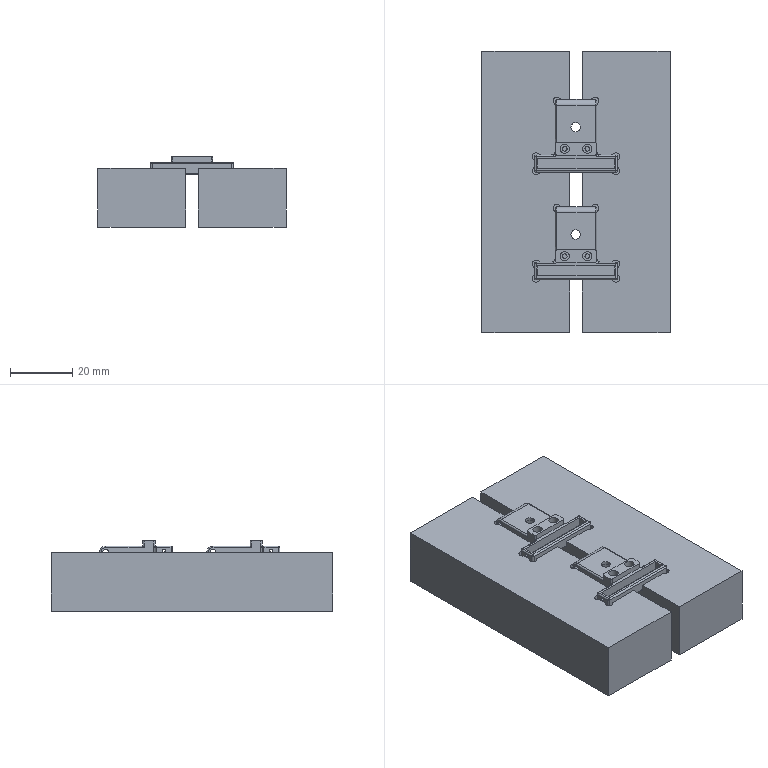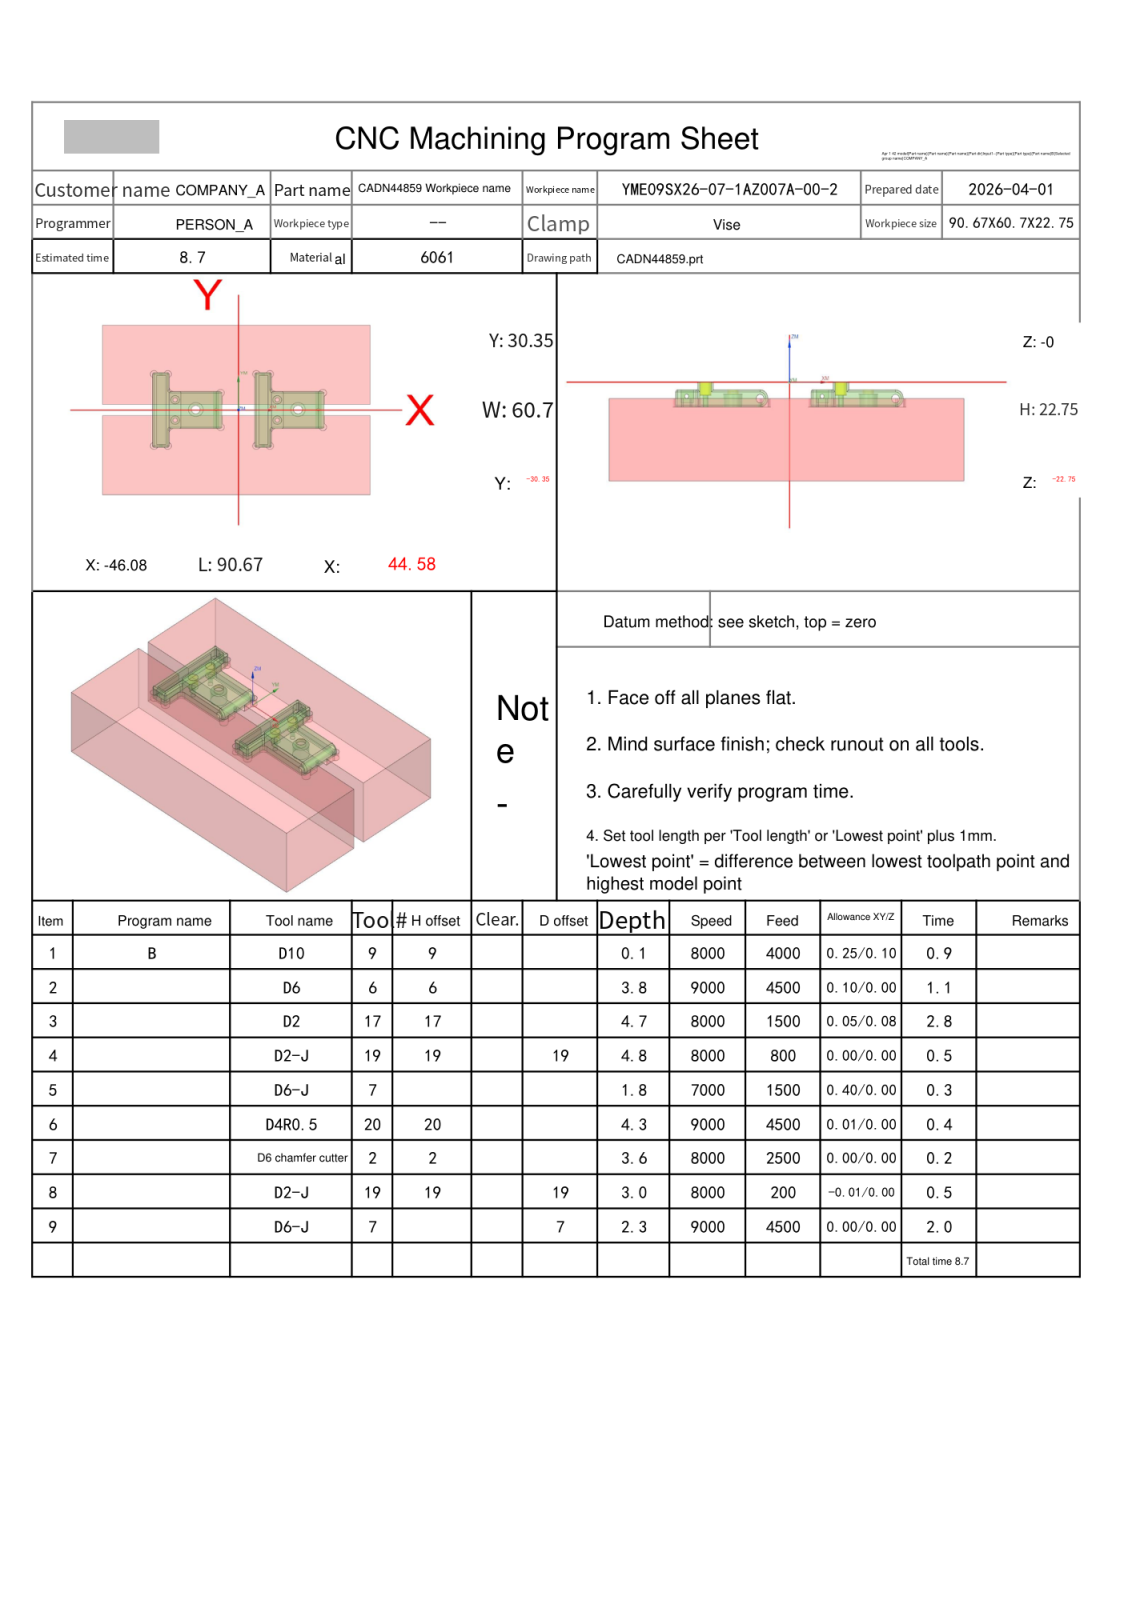NC program | NX | posted by the shop | part box 60.696 x 90.669 x 22.754 mm
Lines 1 to 1599 of 6042:
%
O0001
(Machine time: 10.48 MIN)
(===Total Tool:7===)
(T9=D10     D=10.  R=0.   D-  H09 Z=0.1   )
(T6=D6      D=6.   R=0.   D-  H06 Z=-3.79 )
(T17=D2     D=2.   R=0.   D-  H17 Z=-4.69 )
(T19=D2-J   D=2.   R=0.   D19 H19 Z=-4.75 )
(T7=D6-J    D=6.   R=0.   D-  H00 Z=-2.25 )
(T20=D4R0.5 D=4.   R=0.5  D-  H20 Z=-4.29 )
(T2=D6 chamfer cutter   D=6.   R=0.   D-  H02 Z=-3.55 )
G80 G90 G17 G49 G40
G91 G28 Z0
M01
N1 T09 M06
(D10  D=10. R=0. H=09 ce=0.25 di=0.10)
G00 G90 G54 X-40.842 Y20.381 M03 S8000
G43 H09 Z20.
M08
Z2.1
G01 X-40.747 Y20.349 Z1.476 F4000.
X-40.652 Y20.318 Z1.228
X-40.557 Y20.286 Z1.046
X-40.463 Y20.254 Z.9
X-40.368 Y20.222 Z.777
X-40.273 Y20.19 Z.672
X-40.178 Y20.158 Z.58
X-40.083 Y20.126 Z.5
X-39.989 Y20.094 Z.43
X-39.894 Y20.062 Z.368
X-39.799 Y20.03 Z.314
X-39.704 Y19.999 Z.267
X-39.61 Y19.967 Z.227
X-39.515 Y19.935 Z.192
X-39.42 Y19.903 Z.164
X-39.325 Y19.871 Z.14
X-39.23 Y19.839 Z.123
X-39.136 Y19.807 Z.11
X-39.041 Y19.775 Z.103
X-38.946 Y19.743 Z.1
X-36.729 Y18.997
X-36.569 Y18.972
G03 X-36.315 Y19.038 I0.0 J.518
G02 X-33.516 Y19.957 I3.756 J-6.724
X-26.927 Y20.43 I6.589 J-45.637
X-26.22 Y20.425 I0.0 J-46.111
G01 X30.138 Y20.424
G02 X36.151 Y16.155 I-.263 J-6.74
X37.336 Y10.243 I-16.003 J-6.282
X37.502 Y.85 I-265.863 J-9.393
X37.485 Y-2.174 I-266.029 J0.0
X37.502 Y-6.249 I-476.949 J-4.074
X37.45 Y-13.253 I-476.966 J0.0
X33.27 Y-19.077 I-6.701 J.398
X27.726 Y-20.269 I-6.122 J14.98
X19.91 Y-20.455 I-7.816 J164.512
X18.189 Y-20.446 I0.0 J164.698
G01 X-30.028 Y-20.429
G02 X-36.161 Y-16.157 I.154 J6.76
X-37.332 Y-10.366 I15.734 J6.194
X-37.505 Y-.549 I277.888 J9.817
X-37.485 Y2.832 I278.061 J0.0
X-37.5 Y6.556 I451.277 J3.724
X-37.452 Y13.13 I451.292 J0.0
X-34.138 Y17.894 I6.402 J-.919
X-28.596 Y19.537 I6.567 J-11.986
X-20.913 Y19.853 I7.683 J-93.113
X-19.426 Y19.842 I0.0 J-93.429
G01 X28.403 Y19.826
G02 X35.029 Y15.447 I-.346 J-7.726
X36.613 Y9.328 I-14.784 J-7.091
X36.901 Y.457 I-136.295 J-8.871
X36.882 Y-1.825 I-136.584 J0.0
X36.903 Y-5.413 I-318.323 J-3.588
X36.84 Y-11.719 I-318.344 J0.0
X32.586 Y-17.937 I-7.685 J.693
X26.481 Y-19.565 I-7.111 J14.409
X18.572 Y-19.851 I-7.909 J109.299
X17.188 Y-19.842 I0.0 J109.585
G01 X-28.373 Y-19.827
G02 X-35.024 Y-15.475 I.301 J7.717
X-36.614 Y-9.353 I14.682 J7.081
X-36.897 Y-.811 I128.482 J8.542
X-36.882 Y1.2 I128.765 J0.0
X-36.896 Y4.786 I434.55 J3.585
X-36.851 Y11.095 I434.565 J0.0
X-32.53 Y17.279 I7.805 J-.852
X-26.194 Y18.96 I7.343 J-14.892
X-17.308 Y19.262 I8.886 J-130.709
X-15.161 Y19.244 I0.0 J-131.01
G01 X26.759 Y19.226
G02 X34.346 Y14.205 I-.291 J-8.684
X36.01 Y7.485 I-16.807 J-7.728
X36.295 Y-1.458 I-140.358 J-8.942
X36.281 Y-3.429 I-140.642 J0.0
X36.305 Y-5.816 I-120.556 J-2.387
X36.22 Y-10.327 I-120.58 J0.0
X31.284 Y-17.288 I-8.629 J.888
X24.694 Y-18.957 I-7.673 J16.445
X16.023 Y-19.254 I-8.671 J126.585
X14.321 Y-19.243 I0.0 J126.881
G01 X-26.819 Y-19.224
G02 X-34.337 Y-14.236 I.331 J8.66
X-35.987 Y-7.756 I16.355 J7.615
X-36.287 Y.642 I117.427 J8.398
X-36.278 Y2.077 I117.726 J0.0
X-36.296 Y4.741 I199.73 J2.664
X-36.24 Y9.456 I199.747 J0.0
X-31.263 Y16.631 I8.743 J-.75
X-24.498 Y18.353 I7.851 J-16.702
X-15.886 Y18.651 I8.612 J-124.221
X-14.365 Y18.641 I0.0 J-124.519
G01 X25.094 Y18.63
G02 X33.792 Y12.869 I-.033 J-9.496
X35.393 Y6.07 I-18.671 J-7.984
X35.689 Y-2.856 I-134.771 J-8.926
X35.679 Y-4.483 I-135.066 J0.0
X35.704 Y-5.918 I-41.196 J-1.435
X35.557 Y-9.398 I-41.22 J0.0
X30.113 Y-16.656 I-9.314 J1.315
X23.151 Y-18.352 I-8.101 J18.111
X13.766 Y-18.658 I-9.385 J143.679
X11.698 Y-18.643 I0.0 J143.985
G01 X-25.181 Y-18.627
G02 X-33.711 Y-13.049 I.086 J9.443
X-35.383 Y-6.202 I18.062 J8.037
X-35.69 Y2.818 I132.251 J9.019
X-35.679 Y4.531 I132.558 J0.0
X-35.706 Y5.721 I26.507 J1.19
X-35.477 Y9.199 I26.534 J0.0
X-29.991 Y16.061 I9.358 J-1.857
X-22.967 Y17.751 I8.183 J-18.58
X-13.276 Y18.06 I9.691 J-151.435
X-11.034 Y18.044 I0.0 J-151.744
G01 X23.746 Y18.025
X23.806
G02 X33.198 Y11.714 I0.0 J-10.144
X34.785 Y4.722 I-20.248 J-8.273
X35.081 Y-3.446 I-112.509 J-8.168
X35.006 Y-7.569 I-112.805 J0.0
X29.038 Y-16.028 I-9.98 J.707
X21.957 Y-17.731 I-8.374 J19.249
X12.963 Y-18.047 I-8.995 J127.82
X11.585 Y-18.039 I0.0 J128.136
G01 X-23.854 Y-18.021
G02 X-33.178 Y-11.765 I.026 J10.114
X-34.792 Y-4.658 I20.204 J8.325
X-35.08 Y2.895 I98.916 J7.553
X-34.996 Y6.973 I99.204 J0.0
X-28.872 Y15.46 I10.08 J-.82
X-21.542 Y17.153 I8.509 J-20.134
X-11.764 Y17.457 I9.779 J-156.976
X-9.669 Y17.443 I0.0 J-157.28
G01 X22.411 Y17.423
X22.526 Y17.424
G02 X29.094 Y15.286 I0.0 J-11.159
X33.223 Y8.914 I-7.735 J-9.536
X34.333 Y1.092 I-31.665 J-8.482
X34.457 Y-3.082 I-70.23 J-4.174
X34.37 Y-6.584 I-70.354 J0.0
X28.073 Y-15.382 I-10.446 J.824
X20.694 Y-17.126 I-8.701 J20.336
X11.245 Y-17.449 I-9.449 J138.124
X9.662 Y-17.44 I0.0 J138.447
G01 X-22.298 Y-17.427
X-22.478 Y-17.429
G02 X-28.767 Y-15.53 I0.0 J11.362
X-33.17 Y-9.095 I7.176 J9.635
X-34.322 Y-1.341 I30.345 J8.469
X-34.448 Y2.658 I63.448 J4.
X-34.365 Y5.914 I63.574 J0.0
X-28.047 Y14.754 I10.508 J-.832
X-20.613 Y16.52 I8.772 J-20.399
X-10.524 Y16.857 I10.09 J-150.833
X-8.381 Y16.842 I0.0 J-151.17
G01 X21.119 Y16.823
X21.27 Y16.824
G02 X27.481 Y15.15 I0.0 J-12.36
X32.329 Y8.76 I-6.554 J-10.007
X33.685 Y.738 I-28.136 J-8.88
X33.821 Y-2.613 I-40.982 J-3.351
X33.674 Y-6.094 I-41.118 J0.0
X27.147 Y-14.745 I-10.767 J1.336
X19.709 Y-16.503 I-8.893 J21.002
X9.271 Y-16.859 I-10.437 J153.067
X6.997 Y-16.842 I0.0 J153.422
G01 X-21.123 Y-16.823
X-21.282 Y-16.824
G02 X-27.535 Y-15.119 I0.0 J12.32
X-32.372 Y-8.644 I6.661 J10.019
X-33.689 Y-.677 I28.655 J8.828
X-33.81 Y2.187 I33.686 J2.863
X-33.63 Y5.673 I33.807 J0.0
X-27.198 Y14.086 I10.766 J-1.566
X-19.887 Y15.875 I8.898 J-20.532
X-10.326 Y16.243 I9.56 J-123.703
X-8.976 Y16.236 I0.0 J-124.071
G01 X19.803 Y16.225
G02 X20.034 Y16.227 I.231 J-13.722
X26.069 Y14.829 I0.0 J-13.723
X31.497 Y8.398 I-5.798 J-10.401
X33.02 Y.534 I-25.713 J-9.06
X33.162 Y-2.216 I-26.672 J-2.75
X32.92 Y-5.81 I-26.814 J0.0
X26.456 Y-14.017 I-10.93 J1.96
X18.737 Y-15.886 I-9.21 J21.158
X9.038 Y-16.243 I-9.699 J131.666
X7.706 Y-16.236 I0.0 J132.023
G01 X-19.814 Y-16.225
G02 X-20.043 Y-16.227 I-.229 J13.682
X-26.131 Y-14.798 I0.0 J13.684
X-31.549 Y-8.27 I5.907 J10.415
X-33.034 Y-.337 I26.359 J9.04
X-33.145 Y1.84 I21.233 J2.177
X-32.783 Y5.756 I21.344 J0.0
X-26.29 Y13.463 I10.887 J-2.584
X-18.682 Y15.281 I9.163 J-21.514
X-8.617 Y15.648 I10.065 J-137.713
X-6.931 Y15.638 I0.0 J-138.081
G01 X18.788 Y15.62
X18.969 Y15.621
G02 X25.076 Y14.274 I0.0 J-14.52
X30.864 Y7.541 I-5.713 J-10.764
X32.445 Y-1.785 I-26.711 J-9.326
X32.319 Y-4.455 I-28.292 J0.0
X25.681 Y-13.343 I-11.223 J1.459
X17.911 Y-15.26 I-9.381 J21.327
X7.488 Y-15.651 I-10.423 J138.606
X5.621 Y-15.638 I0.0 J138.997
G01 X-18.539 Y-15.627
G02 X-18.83 Y-15.63 I-.291 J15.256
X-24.739 Y-14.439 I0.0 J15.259
X-30.735 Y-7.872 I5.218 J10.785
X-32.41 Y.927 I24.809 J9.282
X-32.444 Y1.868 I13.077 J.941
X-31.034 Y7.783 I13.111 J0.0
X-24.378 Y13.269 I10.606 J-6.087
X-16.207 Y14.792 I9.315 J-27.292
X-4.645 Y15.063 I11.563 J-246.703
X-1.572 Y15.044 I0.0 J-246.974
G01 X17.548 Y15.023
G02 X17.813 Y15.025 I.265 J-15.892
X23.925 Y13.803 I0.0 J-15.894
X30.063 Y7.135 I-5.288 J-11.028
X31.706 Y-1.466 I-21.699 J-8.601
X31.593 Y-3.761 I-23.341 J0.0
X24.903 Y-12.682 I-11.343 J1.537
X16.957 Y-14.649 I-9.592 J21.709
X6.501 Y-15.047 I-10.456 J137.135
X4.788 Y-15.037 I0.0 J137.533
G01 X-17.452 Y-15.025
G02 X-17.754 Y-15.028 I-.302 J16.286
X-23.73 Y-13.892 I0.0 J16.289
X-30.053 Y-7.166 I5.053 J11.085
X-31.652 Y.994 I20.017 J8.16
X-31.529 Y3.303 I21.616 J0.0
X-25.041 Y11.984 I11.274 J-1.661
X-17.35 Y13.999 I9.538 J-20.728
X-7.318 Y14.436 I10.032 J-114.813
X-6.143 Y14.43 I0.0 J-115.251
G01 X16.336 Y14.425
G02 X16.667 Y14.428 I.33 J-17.538
X22.69 Y13.361 I0.0 J-17.541
X29.351 Y6.525 I-4.821 J-11.36
X30.926 Y-1.13 I-17.821 J-7.655
X30.807 Y-3.277 I-19.396 J0.0
X24.37 Y-11.907 I-11.309 J1.72
X16.58 Y-13.982 I-9.682 J20.688
X6.084 Y-14.442 I-10.496 J119.566
X4.594 Y-14.433 I0.0 J120.025
G01 X-16.506 Y-14.421
G02 X-16.764 Y-14.423 I-.258 J17.012
X-22.847 Y-13.298 I0.0 J17.013
X-29.443 Y-6.312 I5.042 J11.367
X-30.855 Y.679 I16.599 J6.991
X-30.73 Y2.795 I18.011 J0.0
X-24.438 Y11.24 I11.232 J-1.802
X-16.843 Y13.341 I9.643 J-20.081
X-6.81 Y13.828 I10.033 J-103.144
X-5.879 Y13.824 I0.0 J-103.631
G01 X15.341 Y13.823
G02 X15.659 Y13.826 I.318 J-18.556
X21.707 Y12.813 I0.0 J-18.559
X28.697 Y5.798 I-4.657 J-11.63
X30.1 Y-.78 I-14.722 J-6.578
X29.938 Y-3.06 I-16.124 J0.0
X23.757 Y-11.17 I-11.184 J2.113
X15.879 Y-13.349 I-9.845 J20.262
X5.814 Y-13.827 I-10.066 J105.826
X4.975 Y-13.824 I0.0 J106.304
G01 X-15.345 Y-13.823
G02 X-15.682 Y-13.826 I-.337 J18.375
X-21.823 Y-12.77 I0.0 J18.378
X-28.784 Y-5.593 I4.808 J11.627
X-30.009 Y.306 I13.591 J5.899
X-29.796 Y2.807 I14.816 J0.0
X-23.736 Y10.548 I11.07 J-2.424
X-15.917 Y12.735 I9.838 J-20.102
X-5.509 Y13.233 I10.408 J-108.483
X-4.353 Y13.227 I0.0 J-108.981
X4.021 Y13.265 I8.374 J-925.635
X15.186 Y13.197 I0.0 J-925.673
G01 X15.195
G02 X21.944 Y11.749 I0.0 J-16.452
X28.374 Y4.22 I-5.943 J-11.585
X29.232 Y-.388 I-11.945 J-4.608
X28.738 Y-3.909 I-12.803 J0.0
X22.618 Y-10.704 I-10.949 J3.708
X14.879 Y-12.753 I-9.771 J21.262
X4.119 Y-13.239 I-10.761 J118.93
X2.654 Y-13.23 I0.0 J119.415
X-4.535 Y-13.262 I-7.189 J802.826
X-15.385 Y-13.189 I0.0 J802.858
X-22.226 Y-11.611 I.071 J15.92
X-28.521 Y-3.728 I6.265 J11.459
X-29.129 Y-.051 I10.82 J3.677
X-27.888 Y5.128 I11.428 J0.0
X-21.399 Y10.618 I10.749 J-6.125
X-13.201 Y12.309 I9.742 J-26.514
X-1.683 Y12.656 I11.519 J-191.294
X.772 Y12.64 I0.0 J-191.64
X5.509 Y12.662 I4.738 J-506.807
X14.611 Y12.58 I0.0 J-506.829
X21.452 Y10.996 I-.149 J-16.207
X28.278 Y-.353 I-6.021 J-11.349
X28.221 Y-1.568 I-12.847 J0.0
X22.801 Y-9.522 I-10.753 J1.504
X15.317 Y-11.971 I-9.932 J17.692
X5.039 Y-12.609 I-10.277 J82.514
X4.483 Y-12.607 I0.0 J83.152
X-4.187 Y-12.663 I-8.67 J662.713
X-14.576 Y-12.582 I0.0 J662.77
X-21.422 Y-11.014 I.126 J16.28
X-28.135 Y-.012 I5.658 J11.002
X-28.112 Y.741 I12.372 J0.0
X-22.838 Y8.85 I10.6 J-1.125
X-15.195 Y11.377 I10.02 J-17.484
X-4.999 Y12.006 I10.195 J-82.263
X-4.541 Y12.005 I0.0 J-82.893
X3.754 Y12.062 I8.295 J-601.862
X13.678 Y11.98 I0.0 J-601.92
X20.593 Y10.434 I-.129 J-16.815
X27.29 Y-.125 I-5.237 J-10.725
X22.393 Y-8.612 I-10.349 J.315
X15.161 Y-11.245 I-9.928 J16.016
X4.924 Y-11.99 I-10.238 J69.983
G01 X4.638 Y-11.989
G02 X-4.158 Y-12.062 I-8.795 J531.122
X-13.781 Y-11.975 I0.0 J531.194
X-20.632 Y-10.416 I.183 J16.64
X-27.097 Y-.896 I5.051 J10.385
X-27.102 Y-.579 I10.048 J.317
X-22.611 Y7.795 I10.053 J0.0
X-15.323 Y10.6 I9.993 J-15.093
X-5.344 Y11.375 I10.008 J-64.281
X3.706 Y11.461 I9.049 J-474.942
X12.955 Y11.371 I0.0 J-475.029
X19.922 Y9.783 I-.201 J-16.957
X26.123 Y1.478 I-4.843 J-10.083
X26.188 Y.352 I-9.615 J-1.126
X22.273 Y-7.425 I-9.681 J0.0
X15.223 Y-10.455 I-9.993 J13.535
X5.315 Y-11.355 I-10.07 J55.9
X-4.087 Y-11.462 I-9.402 J411.125
X-13.103 Y-11.363 I0.0 J411.232
X-20.166 Y-9.658 I.25 J16.512
X-25.848 Y-2.211 I4.841 J9.585
X-25.963 Y-.747 I9.296 J1.464
X-22.278 Y6.721 I9.411 J0.0
X-15.309 Y9.816 I9.946 J-13.006
X-5.466 Y10.748 I10.064 J-53.816
X3.728 Y10.857 I9.193 J-388.9
X12.173 Y10.765 I0.0 J-389.009
X19.145 Y9.189 I-.242 J-17.281
X24.771 Y2.568 I-4.401 J-9.441
X25.008 Y.514 I-8.794 J-2.054
X21.85 Y-6.346 I-9.031 J0.0
X14.943 Y-9.706 I-9.974 J11.727
X5.593 Y-10.717 I-9.884 J47.637
X-4.049 Y-10.859 I-9.642 J327.373
X-12.405 Y-10.753 I0.0 J327.515
X-19.354 Y-9.081 I.341 J16.698
X-24.54 Y-2.79 I4.311 J8.838
X-24.741 Y-.922 I8.602 J1.868
X-21.75 Y5.689 I8.802 J0.0
X-14.934 Y9.08 I9.882 J-11.318
X-5.707 Y10.11 I9.819 J-46.115
X3.633 Y10.255 I9.34 J-299.509
X11.57 Y10.15 I0.0 J-299.654
X18.473 Y8.542 I-.347 J-17.111
X23.491 Y2.72 I-3.98 J-8.504
X23.732 Y.707 I-8.278 J-2.013
X20.947 Y-5.593 I-8.52 J0.0
X14.349 Y-9.009 I-9.745 J10.742
X5.071 Y-10.101 I-9.874 J43.958
X-4.143 Y-10.249 I-9.214 J285.871
X-11.486 Y-10.155 I0.0 J286.02
X-18.396 Y-8.575 I.289 J17.17
X-23.209 Y-2.934 I3.698 J8.029
X-23.411 Y-1.113 I8.114 J1.821
X-20.733 Y5. I8.316 J0.0
X-14.358 Y8.369 I9.572 J-10.395
X-5.384 Y9.484 I9.704 J-41.439
X3.55 Y9.651 I8.933 J-239.093
X10.933 Y9.537 I0.0 J-239.26
X17.607 Y7.986 I-.425 J-16.96
X22.183 Y2.507 I-3.446 J-7.528
X22.34 Y.917 I-7.971 J-1.59
X19.699 Y-5.079 I-8.128 J0.0
X13.384 Y-8.39 I-9.443 J10.334
X4.408 Y-9.487 I-9.667 J41.811
X-4.002 Y-9.645 I-8.409 J224.814
X-10.889 Y-9.539 I0.0 J224.971
X-17.457 Y-8.046 I.384 J16.876
X-21.902 Y-2.304 I3.166 J7.043
X-21.956 Y-1.371 I8.045 J.934
X-19.067 Y4.83 I8.099 J0.0
X-12.529 Y7.958 I9.367 J-11.184
X-3.292 Y8.923 I9.667 J-47.829
X3.491 Y9.044 I6.783 J-190.133
X10.325 Y8.922 I0.0 J-190.254
X16.706 Y7.425 I-.457 J-16.301
X20.816 Y.993 I-2.978 J-6.432
X20.718 Y-.178 I-7.088 J0.0
X16.608 Y-5.942 I-8.649 J1.82
X9.672 Y-8.333 I-9.188 J15.396
X-.553 Y-9.001 I-10.224 J77.978
X-1.099 Y-8.999 I0.0 J78.645
X-4.513 Y-9.05 I-3.414 J114.654
X-11.114 Y-8.86 I0.0 J114.705
X-16.81 Y-7.327 I.765 J14.189
X-20.366 Y-1.355 I3.235 J5.971
X-19.291 Y2.312 I6.792 J0.0
X-13.928 Y6.567 I8.951 J-5.774
X-6.369 Y8.1 I9.016 J-25.047
X3.439 Y8.437 I9.808 J-142.435
X9.94 Y8.289 I0.0 J-142.772
X15.456 Y6.996 I-.594 J-14.948
X19.127 Y1.132 I-2.849 J-5.864
X18.208 Y-2.206 I-6.52 J0.0
X12.874 Y-6.579 I-8.806 J5.3
X5.133 Y-8.124 I-9.027 J25.063
X-3.88 Y-8.427 I-9.013 J133.874
X-9.858 Y-8.294 I0.0 J134.177
X-15.039 Y-7.136 I.503 J14.42
X-18.567 Y-1.524 I2.7 J5.612
X-17.873 Y1.332 I6.228 J0.0
X-12.919 Y5.817 I8.519 J-4.432
X-5.754 Y7.451 I8.693 J-21.595
X3.404 Y7.823 I9.157 J-112.436
X9.413 Y7.663 I0.0 J-112.809
X14. Y6.588 I-.525 J-12.564
X17.209 Y1.305 I-2.744 J-5.283
X16.643 Y-1.228 I-5.953 J0.0
X11.932 Y-5.752 I-8.274 J3.903
X4.899 Y-7.436 I-8.54 J20.13
X-3.762 Y-7.816 I-8.661 J98.588
X-9.606 Y-7.643 I0.0 J98.968
X-13.651 Y-6.629 I.434 J10.304
X-16.509 Y-1.69 I2.84 J4.94
X-16.074 Y.494 I5.698 J0.0
X-11.6 Y5.088 I8.031 J-3.346
X-4.827 Y6.811 I8.316 J-18.506
X3.427 Y7.203 I8.254 J-86.806
X8.896 Y7.031 I0.0 J-87.197
X12.558 Y6.006 I-.284 J-8.067
X14.983 Y1.452 I-3.065 J-4.554
X14.576 Y-.622 I-5.49 J0.0
X10.101 Y-5.195 I-7.871 J3.227
X3.431 Y-6.841 I-8.101 J18.488
X-3.791 Y-7.192 I-7.222 J74.033
X-9.093 Y-7.003 I0.0 J74.384
X-13.51 Y-4.243 I.183 J5.208
X-14.047 Y-1.774 I5.41 J2.469
X-12.719 Y1.972 I5.947 J0.0
X-7.513 Y5.37 I7.877 J-6.382
X.009 Y6.463 I8.145 J-29.614
X3.613 Y6.581 I3.604 J-54.908
X8.34 Y6.378 I0.0 J-55.026
X12.308 Y1.693 I-.781 J-4.685
X12.247 Y.935 I-4.749 J0.0
X8.739 Y-4.148 I-7.104 J1.152
X2.738 Y-6.11 I-7.62 J13.15
X-3.987 Y-6.551 I-6.725 J51.032
X-7.499 Y-6.431 I0.0 J51.473
X-11.074 Y-2.109 I.825 J4.321
X-11.065 Y-1.832 I4.399 J0.0
X-8.074 Y3.334 I6.666 J-.41
X-2.201 Y5.478 I7.464 J-11.331
X3.652 Y5.91 I5.853 J-39.441
X5.576 Y5.863 I0.0 J-39.872
X8.827 Y2.003 I-.761 J-3.94
G01 X8.829 Y1.855
G02 X6.219 Y-3.232 I-6.262 J0.0
X.521 Y-5.468 I-7.244 J10.083
X-3.307 Y-5.821 I-3.828 J20.554
X-4.077 Y-5.807 I0.0 J20.908
X-6.77 Y-3.254 I.772 J3.51
X-6.998 Y-1.713 I5.091 J1.541
X-4.976 Y2.462 I5.319 J0.0
X.643 Y4.821 I6.839 J-8.415
X4.074 Y1.174 I-.846 J-4.234
G01 X4.093 Y1.056
G03 X4.382 Y.679 I.5 J.084
G01 X6.172 Y-.164 Z.2
X7.689 Y-.878
X7.758 Y-.918
X7.821 Y-.969
X7.874 Y-1.029
X7.917 Y-1.097
X7.949 Y-1.17
X8.122 Y-1.679
X8.141 Y-1.758
X8.148 Y-1.839
X8.141 Y-1.92
X8.122 Y-1.999
X8.09 Y-2.074
X8.046 Y-2.142
X7.991 Y-2.203
X7.928 Y-2.254
X7.857 Y-2.294
X7.78 Y-2.322
X7.7 Y-2.337
X6.28 Y-2.487
X4.312 Y-2.694 Z.1
X4.091 Y-2.718
X3.881 Y-2.788
X3.821 Y-2.831
X3.599 Y-3.017
X3.522 Y-3.081 Z.103
X3.445 Y-3.145 Z.11
X3.368 Y-3.21 Z.123
X3.292 Y-3.274 Z.14
X3.215 Y-3.338 Z.164
X3.138 Y-3.402 Z.192
X3.062 Y-3.466 Z.227
X2.985 Y-3.53 Z.267
X2.908 Y-3.594 Z.314
X2.831 Y-3.658 Z.368
X2.755 Y-3.723 Z.43
X2.678 Y-3.787 Z.5
X2.601 Y-3.851 Z.58
X2.524 Y-3.915 Z.672
X2.448 Y-3.979 Z.777
X2.371 Y-4.043 Z.9
X2.294 Y-4.107 Z1.046
X2.218 Y-4.171 Z1.228
X2.141 Y-4.236 Z1.476
X2.064 Y-4.3 Z2.1
G00 Z20.
G91 G28 Z0.0
M05
M09
G91 G28 Z0.0
M01
N2 T06 M06
(D6  D=6. R=0. H=06 ce=0.10 di=0.10)
G00 G90 G54 X-34.584 Y-12.185 M03 S8000
G43 H06 Z11.95
M08
Z1.086
G01 Z-.414 F3000.
X-31.524
Y15.788
X-21.012
Y13.351
X-17.678 Y10.017
G03 X-19.952 Y10.634 I-2.274 J-3.883
G01 X-22.952
G03 X-24.657 Y10.299 I0.0 J-4.5
G02 X-24.884 Y10.254 I-.227 J.555
X-25.117 Y10.301 I0.0 J.6
G01 X-27.543 Y11.323
G03 X-27.775 Y11.369 I-.233 J-.553
X-28. Y11.326 I0.0 J-.6
G02 X-28.224 Y11.282 I-.225 J.556
X-28.824 Y11.881 I0.0 J.6
G01 Y12.489
G02 X-28.226 Y13.088 I.6 J-.001
G01 X-26.411
G02 X-26.112 Y12.788 I-.001 J-.3
X-26.273 Y12.522 I-.3 J0.0
G01 X-26.445 Y12.43
G03 X-26.754 Y11.92 I.291 J-.525
G01 X-26.835 Y8.552
G02 X-26.907 Y8.281 I-.6 J.015
G03 X-27.452 Y6.134 I3.955 J-2.147
G01 Y-6.134
G03 X-22.952 Y-10.634 I4.5 J0.0
G01 X-19.952
G03 X-17.678 Y-10.017 I0.0 J4.5
G01 X-21.012 Y-13.351
Y-15.788
X-31.524
Y-13.871
G02 X-31.238 Y-13.36 I.6 J0.0
G01 X-29.051 Y-12.02
G03 X-28.795 Y-11.695 I-.314 J.512
G02 X-28.224 Y-11.282 I.57 J-.187
X-27.82 Y-11.439 I0.0 J-.6
G03 X-26.273 Y-12.522 I4.868 J5.305
G02 X-26.112 Y-12.788 I-.139 J-.266
X-26.411 Y-13.088 I-.3 J0.0
G01 X-28.226
G02 X-28.824 Y-12.489 I.001 J.6
G01 Y-12.185
Y-11.881
X-28.836 Y-11.78
X-28.792 Y-11.689
X-34.584 Y-9.714
Z1.086
G00 Z11.95
X-1.516 Y0.0
Z1.086
G01 Z-.414
X-4.576
Y-9.074
X-16.545
G03 X-15.452 Y-6.134 I-3.407 J2.94
G01 Y6.134
G03 X-16.353 Y8.834 I-4.5 J0.0
X-16.709 Y9.012 I-.356 J-.267
G01 X-16.827 Y8.996
X-17.094 Y8.923
G03 X-17.292 Y8.662 I.072 J-.26
G01 X-17.227 Y8.486
G02 X-16.352 Y6.134 I-2.725 J-2.352
G01 Y-6.134
G02 X-19.952 Y-9.734 I-3.6 J0.0
G01 X-22.952
G02 X-26.552 Y-6.134 I0.0 J3.6
G01 Y6.134
G02 X-22.952 Y9.734 I3.6 J0.0
G01 X-19.952
G02 X-17.227 Y8.486 I0.0 J-3.6
G03 X-16.776 Y8.279 I.451 J.389
X-16.215 Y8.675 I0.0 J.596
G02 X-15.65 Y9.074 I.565 J-.201
G01 X-4.576
Y1.821
G02 X-4.842 Y1.322 I-.6 J0.0
G01 X-8.809 Y-1.322
G03 X-9.076 Y-1.821 I.333 J-.499
G01 Y-3.975
G02 X-9.674 Y-4.574 I-.6 J.001
G01 X-10.354
G02 X-10.952 Y-3.975 I.001 J.6
G01 Y3.975
G02 X-10.354 Y4.574 I.6 J-.001
G01 X-9.674
G02 X-9.076 Y3.975 I-.001 J-.6
G01 Y0.0
Y-.5
X-1.516
Z1.086
G00 Z11.95
X-34.584 Y12.185
Z.673
G01 Z-.827
X-31.524
Y15.788
X-21.012
Y13.351
X-17.678 Y10.017
G03 X-19.952 Y10.634 I-2.274 J-3.883
G01 X-22.952
G03 X-27.452 Y6.134 I0.0 J-4.5
G01 Y-6.134
G03 X-22.952 Y-10.634 I4.5 J0.0
G01 X-19.952
G03 X-17.678 Y-10.017 I0.0 J4.5
G01 X-21.012 Y-13.351
Y-15.788
X-31.524
Y-13.602
G02 X-31.193 Y-13.065 I.6 J0.0
G01 X-29.085 Y-12.011
G03 X-28.789 Y-11.678 I-.269 J.537
G02 X-28.224 Y-11.282 I.564 J-.204
X-27.82 Y-11.439 I0.0 J-.6
G03 X-26.273 Y-12.522 I4.868 J5.305
G02 X-26.112 Y-12.788 I-.139 J-.266
X-26.411 Y-13.088 I-.3 J0.0
G01 X-28.226
G02 X-28.799 Y-12.66 I.001 J.6
G03 X-29.022 Y-12.346 I-.575 J-.172
G01 X-31.277 Y-10.711
G02 X-31.524 Y-10.225 I.352 J.486
G01 Y10.225
G02 X-31.277 Y10.711 I.6 J0.0
G01 X-29.022 Y12.346
G03 X-28.799 Y12.66 I-.352 J.486
G02 X-28.226 Y13.088 I.575 J-.172
G01 X-26.411
G02 X-26.112 Y12.788 I-.001 J-.3
X-26.273 Y12.522 I-.3 J0.0
G03 X-27.82 Y11.439 I3.321 J-6.388
G02 X-28.224 Y11.282 I-.405 J.443
X-28.824 Y11.881 I0.0 J.6
G01 Y12.381
X-34.584
Z.673
G00 Z11.95
X-1.516 Y0.0
Z.673
G01 Z-.827
X-4.576
Y-9.074
X-16.545
G03 X-15.452 Y-6.134 I-3.407 J2.94
G01 Y6.134
G03 X-16.353 Y8.834 I-4.5 J0.0
X-16.709 Y9.012 I-.356 J-.267
G01 X-16.827 Y8.996
X-17.094 Y8.923
G03 X-17.292 Y8.662 I.072 J-.26
G01 X-17.227 Y8.486
G02 X-16.352 Y6.134 I-2.725 J-2.352
G01 Y-6.134
G02 X-19.952 Y-9.734 I-3.6 J0.0
G01 X-22.952
G02 X-26.552 Y-6.134 I0.0 J3.6
G01 Y6.134
G02 X-22.952 Y9.734 I3.6 J0.0
G01 X-19.952
G02 X-17.227 Y8.486 I0.0 J-3.6
G03 X-16.776 Y8.279 I.451 J.389
X-16.215 Y8.675 I0.0 J.596
G02 X-15.65 Y9.074 I.565 J-.201
G01 X-4.576
Y1.821
G02 X-4.842 Y1.322 I-.6 J0.0
G01 X-8.809 Y-1.322
G03 X-9.076 Y-1.821 I.333 J-.499
G01 Y-3.975
G02 X-9.674 Y-4.574 I-.6 J.001
G01 X-10.354
G02 X-10.952 Y-3.975 I.001 J.6
G01 Y3.975
G02 X-10.354 Y4.574 I.6 J-.001
G01 X-9.674
G02 X-9.076 Y3.975 I-.001 J-.6
G01 Y0.0
Y-.5
X-1.516
Z.673
G00 Z11.95
X-34.584 Y12.185
Z.259
G01 Z-1.241
X-31.524
Y15.788
X-21.012
Y13.351
X-17.678 Y10.017
G03 X-19.952 Y10.634 I-2.274 J-3.883
G01 X-22.952
G03 X-27.452 Y6.134 I0.0 J-4.5
G01 Y-6.134
G03 X-22.952 Y-10.634 I4.5 J0.0
G01 X-19.952
G03 X-17.678 Y-10.017 I0.0 J4.5
G01 X-21.012 Y-13.351
Y-15.788
X-31.524
Y-13.602
G02 X-31.193 Y-13.065 I.6 J0.0
G01 X-29.085 Y-12.011
G03 X-28.789 Y-11.678 I-.269 J.537
G02 X-28.224 Y-11.282 I.564 J-.204
X-27.82 Y-11.439 I0.0 J-.6
G03 X-26.273 Y-12.522 I4.868 J5.305
G02 X-26.112 Y-12.788 I-.139 J-.266
X-26.411 Y-13.088 I-.3 J0.0
G01 X-28.226
G02 X-28.799 Y-12.66 I.001 J.6
G03 X-29.022 Y-12.346 I-.575 J-.172
G01 X-31.277 Y-10.711
G02 X-31.524 Y-10.225 I.352 J.486
G01 Y10.225
G02 X-31.277 Y10.711 I.6 J0.0
G01 X-29.022 Y12.346
G03 X-28.799 Y12.66 I-.352 J.486
G02 X-28.226 Y13.088 I.575 J-.172
G01 X-26.411
G02 X-26.112 Y12.788 I-.001 J-.3
X-26.273 Y12.522 I-.3 J0.0
G03 X-27.82 Y11.439 I3.321 J-6.388
G02 X-28.224 Y11.282 I-.405 J.443
X-28.824 Y11.881 I0.0 J.6
G01 Y12.381
X-34.584
Z.259
G00 Z11.95
X-1.516 Y0.0
Z.259
G01 Z-1.241
X-4.576
Y-9.074
X-16.545
G03 X-15.452 Y-6.134 I-3.407 J2.94
G01 Y6.134
G03 X-16.353 Y8.834 I-4.5 J0.0
X-16.709 Y9.012 I-.356 J-.267
G01 X-16.827 Y8.996
X-17.094 Y8.923
G03 X-17.292 Y8.662 I.072 J-.26
G01 X-17.227 Y8.486
G02 X-16.352 Y6.134 I-2.725 J-2.352
G01 Y-6.134
G02 X-19.952 Y-9.734 I-3.6 J0.0
G01 X-22.952
G02 X-26.552 Y-6.134 I0.0 J3.6
G01 Y6.134
G02 X-22.952 Y9.734 I3.6 J0.0
G01 X-19.952
G02 X-17.227 Y8.486 I0.0 J-3.6
G03 X-16.776 Y8.279 I.451 J.389
X-16.215 Y8.675 I0.0 J.596
G02 X-15.65 Y9.074 I.565 J-.201
G01 X-4.576
Y1.821
G02 X-4.842 Y1.322 I-.6 J0.0
G01 X-8.809 Y-1.322
G03 X-9.076 Y-1.821 I.333 J-.499
G01 Y-3.975
G02 X-9.674 Y-4.574 I-.6 J.001
G01 X-10.354
G02 X-10.952 Y-3.975 I.001 J.6
G01 Y3.975
G02 X-10.354 Y4.574 I.6 J-.001
G01 X-9.674
G02 X-9.076 Y3.975 I-.001 J-.6
G01 Y0.0
Y-.5
X-1.516
Z.259
G00 Z11.95
X-34.584 Y12.185
Z-.154
G01 Z-1.654
X-31.524
Y15.788
X-21.012
Y13.351
X-17.678 Y10.017
G03 X-19.952 Y10.634 I-2.274 J-3.883
G01 X-22.952
G03 X-27.452 Y6.134 I0.0 J-4.5
G01 Y-6.134
G03 X-22.952 Y-10.634 I4.5 J0.0
G01 X-19.952
G03 X-17.678 Y-10.017 I0.0 J4.5
G01 X-21.012 Y-13.351
Y-15.788
X-31.524
Y-13.602
G02 X-31.193 Y-13.065 I.6 J0.0
G01 X-29.085 Y-12.011
G03 X-28.789 Y-11.678 I-.269 J.537
G02 X-28.224 Y-11.282 I.564 J-.204
X-27.82 Y-11.439 I0.0 J-.6
G03 X-26.273 Y-12.522 I4.868 J5.305
G02 X-26.112 Y-12.788 I-.139 J-.266
X-26.411 Y-13.088 I-.3 J0.0
G01 X-28.226
G02 X-28.799 Y-12.66 I.001 J.6
G03 X-29.022 Y-12.346 I-.575 J-.172
G01 X-31.277 Y-10.711
G02 X-31.524 Y-10.225 I.352 J.486
G01 Y10.225
G02 X-31.277 Y10.711 I.6 J0.0
G01 X-29.022 Y12.346
G03 X-28.799 Y12.66 I-.352 J.486
G02 X-28.226 Y13.088 I.575 J-.172
G01 X-26.411
G02 X-26.112 Y12.788 I-.001 J-.3
X-26.273 Y12.522 I-.3 J0.0
G03 X-27.82 Y11.439 I3.321 J-6.388
G02 X-28.224 Y11.282 I-.405 J.443
X-28.824 Y11.881 I0.0 J.6
G01 Y12.381
X-34.584
Z-.154
G00 Z11.95
X-1.516 Y0.0
Z-.154
G01 Z-1.654
X-4.576
Y-9.074
X-16.545
G03 X-15.452 Y-6.134 I-3.407 J2.94
G01 Y6.134
G03 X-16.353 Y8.834 I-4.5 J0.0
X-16.709 Y9.012 I-.356 J-.267
G01 X-16.827 Y8.996
X-17.094 Y8.923
G03 X-17.292 Y8.662 I.072 J-.26
G01 X-17.227 Y8.486
G02 X-16.352 Y6.134 I-2.725 J-2.352
G01 Y-6.134
G02 X-19.952 Y-9.734 I-3.6 J0.0
G01 X-22.952
G02 X-26.552 Y-6.134 I0.0 J3.6
G01 Y6.134
G02 X-22.952 Y9.734 I3.6 J0.0
G01 X-19.952
G02 X-17.227 Y8.486 I0.0 J-3.6
G03 X-16.776 Y8.279 I.451 J.389
X-16.215 Y8.675 I0.0 J.596
G02 X-15.65 Y9.074 I.565 J-.201
G01 X-4.576
Y1.821
G02 X-4.842 Y1.322 I-.6 J0.0
G01 X-8.809 Y-1.322
G03 X-9.076 Y-1.821 I.333 J-.499
G01 Y-3.975
G02 X-9.674 Y-4.574 I-.6 J.001
G01 X-10.354
G02 X-10.952 Y-3.975 I.001 J.6
G01 Y3.975
G02 X-10.354 Y4.574 I.6 J-.001
G01 X-9.674
G02 X-9.076 Y3.975 I-.001 J-.6
G01 Y0.0
Y-.5
X-1.516
Z-.154
G00 Z3.
X.016 Y12.185
Z1.086
G01 Z-.414
X3.076
Y15.788
X13.588
Y13.351
X16.922 Y10.017
G03 X14.648 Y10.634 I-2.274 J-3.883
G01 X11.648
G03 X7.148 Y6.134 I0.0 J-4.5
G01 Y-6.134
G03 X11.648 Y-10.634 I4.5 J0.0
G01 X14.648
G03 X16.922 Y-10.017 I0.0 J4.5
G01 X13.588 Y-13.351
Y-15.788
X3.076
Y-13.602
G02 X3.407 Y-13.065 I.6 J0.0
G01 X5.515 Y-12.011
G03 X5.811 Y-11.678 I-.269 J.537
G02 X6.376 Y-11.282 I.564 J-.204
X6.78 Y-11.439 I0.0 J-.6
G03 X8.327 Y-12.522 I4.868 J5.305
G02 X8.488 Y-12.788 I-.139 J-.266
X8.189 Y-13.088 I-.3 J0.0
G01 X6.374
G02 X5.801 Y-12.66 I.001 J.6
G03 X5.578 Y-12.346 I-.575 J-.172
G01 X3.323 Y-10.711
G02 X3.076 Y-10.225 I.352 J.486
G01 Y10.225
G02 X3.323 Y10.711 I.6 J0.0
G01 X5.578 Y12.346
G03 X5.801 Y12.66 I-.352 J.486
G02 X6.374 Y13.088 I.575 J-.172
G01 X8.189
G02 X8.488 Y12.788 I-.001 J-.3
X8.327 Y12.522 I-.3 J0.0
G03 X6.78 Y11.439 I3.321 J-6.388
G02 X6.376 Y11.282 I-.405 J.443
X5.776 Y11.881 I0.0 J.6
G01 Y12.381
X.016
Z1.086
G00 Z11.95
X33.084 Y0.0
Z1.086
G01 Z-.414
X30.024
Y-9.074
X18.055
G03 X19.148 Y-6.134 I-3.407 J2.94
G01 Y6.134
G03 X18.247 Y8.834 I-4.5 J0.0
X17.891 Y9.012 I-.356 J-.267
G01 X17.773 Y8.996
X17.506 Y8.923
G03 X17.308 Y8.662 I.072 J-.26
G01 X17.373 Y8.486
G02 X18.248 Y6.134 I-2.725 J-2.352
G01 Y-6.134
G02 X14.648 Y-9.734 I-3.6 J0.0
G01 X11.648
G02 X8.048 Y-6.134 I0.0 J3.6
G01 Y6.134
G02 X11.648 Y9.734 I3.6 J0.0
G01 X14.648
G02 X17.373 Y8.486 I0.0 J-3.6
G03 X17.824 Y8.279 I.451 J.389
X18.385 Y8.675 I0.0 J.596
G02 X18.95 Y9.074 I.565 J-.201
G01 X30.024
Y1.821
G02 X29.758 Y1.322 I-.6 J0.0
G01 X25.791 Y-1.322
G03 X25.524 Y-1.821 I.333 J-.499
G01 Y-3.975
G02 X24.926 Y-4.574 I-.6 J.001
G01 X24.246
G02 X23.648 Y-3.975 I.001 J.6
G01 Y3.975
G02 X24.246 Y4.574 I.6 J-.001
G01 X24.926
G02 X25.524 Y3.975 I-.001 J-.6
G01 Y0.0
Y-.5
X33.084
Z1.086
G00 Z11.95
X.016 Y12.185
Z.673
G01 Z-.827
X3.076
Y15.788
X13.588
Y13.351
X16.922 Y10.017
G03 X14.648 Y10.634 I-2.274 J-3.883
G01 X11.648
G03 X7.148 Y6.134 I0.0 J-4.5
G01 Y-6.134
G03 X11.648 Y-10.634 I4.5 J0.0
G01 X14.648
G03 X16.922 Y-10.017 I0.0 J4.5
G01 X13.588 Y-13.351
Y-15.788
X3.076
Y-13.602
G02 X3.407 Y-13.065 I.6 J0.0
G01 X5.515 Y-12.011
G03 X5.811 Y-11.678 I-.269 J.537
G02 X6.376 Y-11.282 I.564 J-.204
X6.78 Y-11.439 I0.0 J-.6
G03 X8.327 Y-12.522 I4.868 J5.305
G02 X8.488 Y-12.788 I-.139 J-.266
X8.189 Y-13.088 I-.3 J0.0
G01 X6.374
G02 X5.801 Y-12.66 I.001 J.6
G03 X5.578 Y-12.346 I-.575 J-.172
G01 X3.323 Y-10.711
G02 X3.076 Y-10.225 I.352 J.486
G01 Y10.225
G02 X3.323 Y10.711 I.6 J0.0
G01 X5.578 Y12.346
G03 X5.801 Y12.66 I-.352 J.486
G02 X6.374 Y13.088 I.575 J-.172
G01 X8.189
G02 X8.488 Y12.788 I-.001 J-.3
X8.327 Y12.522 I-.3 J0.0
G03 X6.78 Y11.439 I3.321 J-6.388
G02 X6.376 Y11.282 I-.405 J.443
X5.776 Y11.881 I0.0 J.6
G01 Y12.381
X.016
Z.673
G00 Z11.95
X33.084 Y0.0
Z.673
G01 Z-.827
X30.024
Y-9.074
X18.055
G03 X19.148 Y-6.134 I-3.407 J2.94
G01 Y6.134
G03 X18.247 Y8.834 I-4.5 J0.0
X17.891 Y9.012 I-.356 J-.267
G01 X17.773 Y8.996
X17.506 Y8.923
G03 X17.308 Y8.662 I.072 J-.26
G01 X17.373 Y8.486
G02 X18.248 Y6.134 I-2.725 J-2.352
G01 Y-6.134
G02 X14.648 Y-9.734 I-3.6 J0.0
G01 X11.648
G02 X8.048 Y-6.134 I0.0 J3.6
G01 Y6.134
G02 X11.648 Y9.734 I3.6 J0.0
G01 X14.648
G02 X17.373 Y8.486 I0.0 J-3.6
G03 X17.824 Y8.279 I.451 J.389
X18.385 Y8.675 I0.0 J.596
G02 X18.95 Y9.074 I.565 J-.201
G01 X30.024
Y1.821
G02 X29.758 Y1.322 I-.6 J0.0
G01 X25.791 Y-1.322
G03 X25.524 Y-1.821 I.333 J-.499
G01 Y-3.975
G02 X24.926 Y-4.574 I-.6 J.001
G01 X24.246
G02 X23.648 Y-3.975 I.001 J.6
G01 Y3.975
G02 X24.246 Y4.574 I.6 J-.001
G01 X24.926
G02 X25.524 Y3.975 I-.001 J-.6
G01 Y0.0
Y-.5
X33.084
Z.673
G00 Z11.95
X.016 Y12.185
Z.259
G01 Z-1.241
X3.076
Y15.788
X13.588
Y13.351
X16.922 Y10.017
G03 X14.648 Y10.634 I-2.274 J-3.883
G01 X11.648
G03 X7.148 Y6.134 I0.0 J-4.5
G01 Y-6.134
G03 X11.648 Y-10.634 I4.5 J0.0
G01 X14.648
G03 X16.922 Y-10.017 I0.0 J4.5
G01 X13.588 Y-13.351
Y-15.788
X3.076
Y-13.602
G02 X3.407 Y-13.065 I.6 J0.0
G01 X5.515 Y-12.011
G03 X5.811 Y-11.678 I-.269 J.537
G02 X6.376 Y-11.282 I.564 J-.204
X6.78 Y-11.439 I0.0 J-.6
G03 X8.327 Y-12.522 I4.868 J5.305
G02 X8.488 Y-12.788 I-.139 J-.266
X8.189 Y-13.088 I-.3 J0.0
G01 X6.374
G02 X5.801 Y-12.66 I.001 J.6
G03 X5.578 Y-12.346 I-.575 J-.172
G01 X3.323 Y-10.711
G02 X3.076 Y-10.225 I.352 J.486
G01 Y10.225
G02 X3.323 Y10.711 I.6 J0.0
G01 X5.578 Y12.346
G03 X5.801 Y12.66 I-.352 J.486
G02 X6.374 Y13.088 I.575 J-.172
G01 X8.189
G02 X8.488 Y12.788 I-.001 J-.3
X8.327 Y12.522 I-.3 J0.0
G03 X6.78 Y11.439 I3.321 J-6.388
G02 X6.376 Y11.282 I-.405 J.443
X5.776 Y11.881 I0.0 J.6
G01 Y12.381
X.016
Z.259
G00 Z11.95
X33.084 Y0.0
Z.259
G01 Z-1.241
X30.024
Y-9.074
X18.055
G03 X19.148 Y-6.134 I-3.407 J2.94
G01 Y6.134
G03 X18.247 Y8.834 I-4.5 J0.0
X17.891 Y9.012 I-.356 J-.267
G01 X17.773 Y8.996
X17.506 Y8.923
G03 X17.308 Y8.662 I.072 J-.26
G01 X17.373 Y8.486
G02 X18.248 Y6.134 I-2.725 J-2.352
G01 Y-6.134
G02 X14.648 Y-9.734 I-3.6 J0.0
G01 X11.648
G02 X8.048 Y-6.134 I0.0 J3.6
G01 Y6.134
G02 X11.648 Y9.734 I3.6 J0.0
G01 X14.648
G02 X17.373 Y8.486 I0.0 J-3.6
G03 X17.824 Y8.279 I.451 J.389
X18.385 Y8.675 I0.0 J.596
G02 X18.95 Y9.074 I.565 J-.201
G01 X30.024
Y1.821
G02 X29.758 Y1.322 I-.6 J0.0
G01 X25.791 Y-1.322
G03 X25.524 Y-1.821 I.333 J-.499
G01 Y-3.975
G02 X24.926 Y-4.574 I-.6 J.001
G01 X24.246
G02 X23.648 Y-3.975 I.001 J.6
G01 Y3.975
G02 X24.246 Y4.574 I.6 J-.001
G01 X24.926
G02 X25.524 Y3.975 I-.001 J-.6
G01 Y0.0
Y-.5
X33.084
Z.259
G00 Z11.95
X.016 Y12.185
Z-.154
G01 Z-1.654
X3.076
Y15.788
X13.588
Y13.351
X16.922 Y10.017
G03 X14.648 Y10.634 I-2.274 J-3.883
G01 X11.648
G03 X7.148 Y6.134 I0.0 J-4.5
G01 Y-6.134
G03 X11.648 Y-10.634 I4.5 J0.0
G01 X14.648
G03 X16.922 Y-10.017 I0.0 J4.5
G01 X13.588 Y-13.351
Y-15.788
X3.076
Y-13.602
G02 X3.407 Y-13.065 I.6 J0.0
G01 X5.515 Y-12.011
G03 X5.811 Y-11.678 I-.269 J.537
G02 X6.376 Y-11.282 I.564 J-.204
X6.78 Y-11.439 I0.0 J-.6
G03 X8.327 Y-12.522 I4.868 J5.305
G02 X8.488 Y-12.788 I-.139 J-.266
X8.189 Y-13.088 I-.3 J0.0
G01 X6.374
G02 X5.801 Y-12.66 I.001 J.6
G03 X5.578 Y-12.346 I-.575 J-.172
G01 X3.323 Y-10.711
G02 X3.076 Y-10.225 I.352 J.486
G01 Y10.225
G02 X3.323 Y10.711 I.6 J0.0
G01 X5.578 Y12.346
G03 X5.801 Y12.66 I-.352 J.486
G02 X6.374 Y13.088 I.575 J-.172
G01 X8.189
G02 X8.488 Y12.788 I-.001 J-.3
X8.327 Y12.522 I-.3 J0.0
G03 X6.78 Y11.439 I3.321 J-6.388
G02 X6.376 Y11.282 I-.405 J.443
X5.776 Y11.881 I0.0 J.6
G01 Y12.381
X.016
Z-.154
G00 Z11.95
X33.084 Y0.0
Z-.154
G01 Z-1.654
X30.024
Y-9.074
X18.055
G03 X19.148 Y-6.134 I-3.407 J2.94
G01 Y6.134
G03 X18.247 Y8.834 I-4.5 J0.0
X17.891 Y9.012 I-.356 J-.267
G01 X17.773 Y8.996
X17.506 Y8.923
G03 X17.308 Y8.662 I.072 J-.26
G01 X17.373 Y8.486
G02 X18.248 Y6.134 I-2.725 J-2.352
G01 Y-6.134
G02 X14.648 Y-9.734 I-3.6 J0.0
G01 X11.648
G02 X8.048 Y-6.134 I0.0 J3.6
G01 Y6.134
G02 X11.648 Y9.734 I3.6 J0.0
G01 X14.648
G02 X17.373 Y8.486 I0.0 J-3.6
G03 X17.824 Y8.279 I.451 J.389
X18.385 Y8.675 I0.0 J.596
G02 X18.95 Y9.074 I.565 J-.201
G01 X30.024
Y1.821
G02 X29.758 Y1.322 I-.6 J0.0
G01 X25.791 Y-1.322
G03 X25.524 Y-1.821 I.333 J-.499
G01 Y-3.975
G02 X24.926 Y-4.574 I-.6 J.001
G01 X24.246
G02 X23.648 Y-3.975 I.001 J.6
G01 Y3.975
G02 X24.246 Y4.574 I.6 J-.001
G01 X24.926
G02 X25.524 Y3.975 I-.001 J-.6
G01 Y0.0
Y-.5
X33.084
Z-.154
G00 Z11.95
G00 G90 X23.096 Y12.38 M03 S9000
Z11.95
Z-1.276
G01 Z-1.776 F4500.
Y12.378
G03 X25.973 Y9.38 I3. J0.0
G01 X27.424 Y9.321
G02 X30.48 Y6.137 I-.131 J-3.184
G01 Y-6.135
G02 X27.421 Y-9.321 I-3.189 J0.0
G01 X25.973 Y-9.38
X25.979 Y-9.437 Z-1.797
X25.983 Y-9.479 Z-1.818
G03 X26.559 Y-9.503 I.576 J7.051
X28.076 Y-9.338 I0.0 J7.075
X30.688 Y-6.134 I-.748 J3.277
G01 Y6.134
G03 X28.076 Y9.338 I-3.359 J-.071
X26.559 Y9.503 I-1.517 J-6.909
X25.983 Y9.479 I0.0 J-7.073
G01 Y9.527 Z-1.849
Y9.566 Z-1.88
G02 X26.537 Y9.582 I.554 J-9.44
X27.999 Y9.468 I0.0 J-9.456
X30.884 Y6.134 I-.616 J-3.448
G01 Y-6.134
G02 X27.999 Y-9.468 I-3.501 J.113
X26.537 Y-9.582 I-1.462 J9.342
X25.983 Y-9.566 I0.0 J9.456
G01 Y-9.606 Z-1.92
Y-9.638 Z-1.96
G03 X26.506 Y-9.648 I.523 J14.044
X27.726 Y-9.595 I0.0 J14.054
X29.947 Y-8.621 I-.414 J3.963
X31.069 Y-6.135 I-2.192 J2.486
G01 Y6.134
G03 X30.825 Y7.364 I-3.626 J-.079
X27.937 Y9.561 I-3.356 J-1.415
X26.526 Y9.652 I-1.411 J-10.9
X25.983 Y9.638 I0.0 J-10.991
G01 Y9.67 Z-2.009
Y9.693 Z-2.057
G02 X26.535 Y9.703 I.552 J-16.68
X27.726 Y9.66 I0.0 J-16.69
X29.483 Y9.118 I-.391 J-4.387
X31.243 Y6.134 I-1.735 J-3.034
G01 Y-6.134
G02 X29.479 Y-9.121 I-3.496 J.051
X27.726 Y-9.66 I-2.143 J3.847
X26.535 Y-9.703 I-1.19 J16.647
X25.983 Y-9.693 I0.0 J16.69
G01 Y-9.727 Z-2.17
X25.994 Y-9.721
G03 X26.526 Y-9.726 I.531 J31.978
X27.726 Y-9.703 I0.0 J31.982
X29.68 Y-9.118 I-.216 J4.276
X31.405 Y-6.134 I-1.792 J3.026
G01 Y6.134
G03 X30.175 Y8.767 I-3.535 J-.048
X27.726 Y9.703 I-2.643 J-3.244
X26.529 Y9.726 I-1.197 J-31.661
X25.994 Y9.721 I0.0 J-31.684
G01 X25.983 Y9.727
X25.989 Y9.733 Z-2.3
G02 X26.55 Y9.736 I.561 J-70.019
X27.726 Y9.726 I0.0 J-70.021
X29.479 Y9.328 I-.059 J-4.316
X31.558 Y6.134 I-1.485 J-3.24
G01 Y-6.134
G02 X29.479 Y-9.328 I-3.564 J.047
X27.726 Y-9.726 I-1.807 J3.899
X26.542 Y-9.735 I-1.184 J72.655
X25.989 Y-9.733 I0.0 J72.665
G01 Z-2.445
X27.726
X28.076 Y-9.722
G03 X29.829 Y-9.236 I-.15 J3.944
X31.697 Y-6.134 I-1.7 J3.136
G01 Y6.134
G03 X30.531 Y8.736 I-3.553 J-.03
X28.076 Y9.723 I-2.592 J-2.897
G01 X27.726 Y9.733
X25.989
Z-2.603
X28.076
G02 X30.18 Y9.116 I-.006 J-3.917
X31.82 Y6.134 I-1.949 J-3.014
G01 Y-6.134
G02 X29.486 Y-9.468 I-3.599 J.035
X28.076 Y-9.733 I-1.438 J3.77
G01 X25.989
Z-2.772
X28.2
G03 X29.489 Y-9.518 I0.0 J3.973
X31.927 Y-6.134 I-1.171 J3.414
G01 Y6.134
G03 X31.552 Y7.715 I-3.706 J-.045
X28.427 Y9.724 I-3.279 J-1.665
G01 X28.076 Y9.733
X25.989
Z-2.951
X28.427
G02 X31.643 Y7.715 I-.059 J-3.666
X32.016 Y6.134 I-3.306 J-1.615
G01 Y-6.134
G02 X29.738 Y-9.468 I-3.625 J.031
X28.366 Y-9.733 I-1.373 J3.431
G01 X25.989
Z-3.138
X28.427
G03 X29.128 Y-9.669 I0.0 J3.88
X32.087 Y-6.134 I-.653 J3.553
G01 Y6.134
G03 X28.464 Y9.733 I-3.624 J-.024
G01 X28.427
X25.989 Y9.734
Z-3.302
X28.427 Y9.733
X28.508 Y9.734
G02 X31.835 Y7.557 I0.0 J-3.631
X32.133 Y6.134 I-3.257 J-1.423
G01 Y-6.134
G02 X29.177 Y-9.666 I-3.588 J0.0
X28.427 Y-9.733 I-.752 J4.198
G01 X25.989
Y-9.734 Z-3.465
X28.439
G03 X28.778 Y-9.723 I0.0 J5.477
X32.164 Y-6.134 I-.223 J3.602
G01 Y6.134
G03 X28.778 Y9.724 I-3.61 J-.013
G01 X28.427 Y9.733
X25.989 Y9.734
Z-3.628
X28.427
X28.778 Y9.727
G02 X32.181 Y6.134 I-.213 J-3.61
G01 Y-6.134
G02 X28.778 Y-9.727 I-3.616 J.016
G01 X28.427 Y-9.734
X25.989
Z-3.792
X28.579
G03 X32.185 Y-6.128 I0.0 J3.606
G01 Y-6.112
X32.184 Y-5.962
Y6.134
G03 X28.585 Y9.734 I-3.599 J0.0
G01 X25.989
G00 Z11.95
X-11.511 Y12.38
Z-1.276
G01 Z-1.776
Y12.378
G03 X-8.633 Y9.38 I3. J0.0
G01 X-7.18 Y9.322
G02 X-4.12 Y6.135 I-.129 J-3.186
G01 Y-6.138
G02 X-7.177 Y-9.322 I-3.186 J0.0
G01 X-8.633 Y-9.38
X-8.626 Y-9.437 Z-1.797
X-8.622 Y-9.479 Z-1.818
X-7.406 Y-9.477
X-7.149 Y-9.461
G03 X-3.912 Y-6.134 I-.206 J3.439
G01 Y6.134
G03 X-7.403 Y9.481 I-3.491 J-.147
G01 X-7.516 Y9.479
X-8.622
Y9.527 Z-1.849
Y9.566 Z-1.88
G02 X-8.07 Y9.582 I.552 J-9.251
X-6.53 Y9.454 I0.0 J-9.268
X-3.716 Y6.134 I-.68 J-3.429
G01 Y-6.134
G02 X-6.53 Y-9.454 I-3.494 J.109
X-8.072 Y-9.582 I-1.542 J9.175
X-8.622 Y-9.566 I0.0 J9.304
G01 Y-9.606 Z-1.92
Y-9.638 Z-1.96
G03 X-8.118 Y-9.647 I.504 J15.081
X-7.005 Y-9.606 I0.0 J15.09
X-4.689 Y-8.651 I-.296 J4.004
X-3.531 Y-6.134 I-2.156 J2.517
G01 Y6.134
G03 X-3.775 Y7.364 I-3.591 J-.073
X-6.53 Y9.543 I-3.366 J-1.425
X-8.075 Y9.652 I-1.545 J-10.925
X-8.622 Y9.638 I0.0 J-11.034
G01 Y9.67 Z-2.009
Y9.693 Z-2.057
G02 X-8.069 Y9.702 I.553 J-16.9
X-6.881 Y9.661 I0.0 J-16.909
X-5.118 Y9.118 I-.384 J-4.38
X-3.357 Y6.134 I-1.731 J-3.033
G01 Y-6.134
G02 X-5.129 Y-9.124 I-3.494 J.05
X-6.881 Y-9.661 I-2.135 J3.845
X-8.084 Y-9.702 I-1.203 J17.648
X-8.622 Y-9.693 I0.0 J17.689
G01 Y-9.727 Z-2.17
X-8.611 Y-9.721
G03 X-8.083 Y-9.726 I.528 J33.059
X-6.881 Y-9.704 I0.0 J33.064
X-5.129 Y-9.235 I-.238 J4.402
X-3.195 Y-6.134 I-1.596 J3.149
G01 Y6.134
G03 X-4.424 Y8.767 I-3.541 J-.05
X-6.881 Y9.704 I-2.646 J-3.251
X-8.077 Y9.726 I-1.196 J-32.448
X-8.611 Y9.721 I0.0 J-32.47
G01 X-8.622 Y9.727
X-8.616 Y9.733 Z-2.3
G02 X-8.135 Y9.735 I.482 J-91.819
X-6.881 Y9.726 I0.0 J-91.82
X-4.733 Y9.118 I-.036 J-4.221
X-3.042 Y6.134 I-1.863 J-3.026
G01 Y-6.134
G02 X-5.129 Y-9.331 I-3.565 J.047
X-6.881 Y-9.726 I-1.803 J3.916
X-8.136 Y-9.735 I-1.255 J92.087
X-8.616 Y-9.733 I0.0 J92.095
G01 Z-2.445
X-6.775
G03 X-5.251 Y-9.46 I0.0 J4.39
X-2.903 Y-6.134 I-1.249 J3.373
G01 Y6.134
G03 X-4.569 Y9.118 I-3.577 J-.04
X-6.53 Y9.724 I-2.116 J-3.37
G01 X-6.881 Y9.733
X-8.616
Z-2.603
X-6.53
X-6.522
G02 X-4.077 Y8.866 I0.0 J-3.881
X-2.78 Y6.134 I-2.295 J-2.764
G01 Y-6.134
G02 X-5.113 Y-9.468 I-3.597 J.033
X-6.53 Y-9.733 I-1.439 J3.78
G01 X-8.616
Z-2.772
X-6.401
G03 X-5.122 Y-9.522 I0.0 J3.982
X-2.673 Y-6.134 I-1.159 J3.417
G01 Y6.134
G03 X-3.048 Y7.715 I-3.675 J-.037
X-6.18 Y9.725 I-3.28 J-1.667
G01 X-6.53 Y9.733
X-8.616
Z-2.951
X-6.18
G02 X-2.956 Y7.715 I-.052 J-3.666
X-2.584 Y6.134 I-3.302 J-1.613
G01 Y-6.134
G02 X-5.129 Y-9.56 I-3.606 J.02
X-6.18 Y-9.733 I-1.137 J3.631
G01 X-8.616
Z-3.138
X-6.178
G03 X-5.479 Y-9.67 I0.0 J3.919
X-2.513 Y-6.134 I-.644 J3.553
G01 Y6.134
G03 X-6.137 Y9.734 I-3.625 J-.025
G01 X-6.18 Y9.733
X-8.616
Z-3.302
X-6.18
X-5.829 Y9.72
G02 X-2.467 Y6.134 I-.243 J-3.596
G01 Y-6.135
G02 X-5.399 Y-9.663 I-3.589 J0.0
X-6.161 Y-9.733 I-.762 J4.09
G01 X-6.18
X-8.616
Y-9.734 Z-3.465
X-6.18 Y-9.733
X-5.829 Y-9.725
G03 X-2.436 Y-6.134 I-.217 J3.603
G01 Y6.134
G03 X-5.829 Y9.725 I-3.61 J-.013
G01 X-6.18 Y9.733
X-8.616 Y9.734
Z-3.628
X-6.028
G02 X-2.427 Y6.218 I0.0 J-3.602
G01 X-2.425 Y6.144
X-2.419 Y6.134
Y-6.134
X-2.425 Y-6.147
X-2.427 Y-6.219
G02 X-6.027 Y-9.734 I-3.601 J.087
G01 X-8.616
Z-3.792
X-6.015
G03 X-2.415 Y-6.134 I0.0 J3.6
G01 Y6.134
G03 X-6.015 Y9.734 I-3.6 J0.0
G01 X-8.616
G00 Z11.95
G91 G28 Z0.0
M05
M09
G91 G28 Z0.0
M01